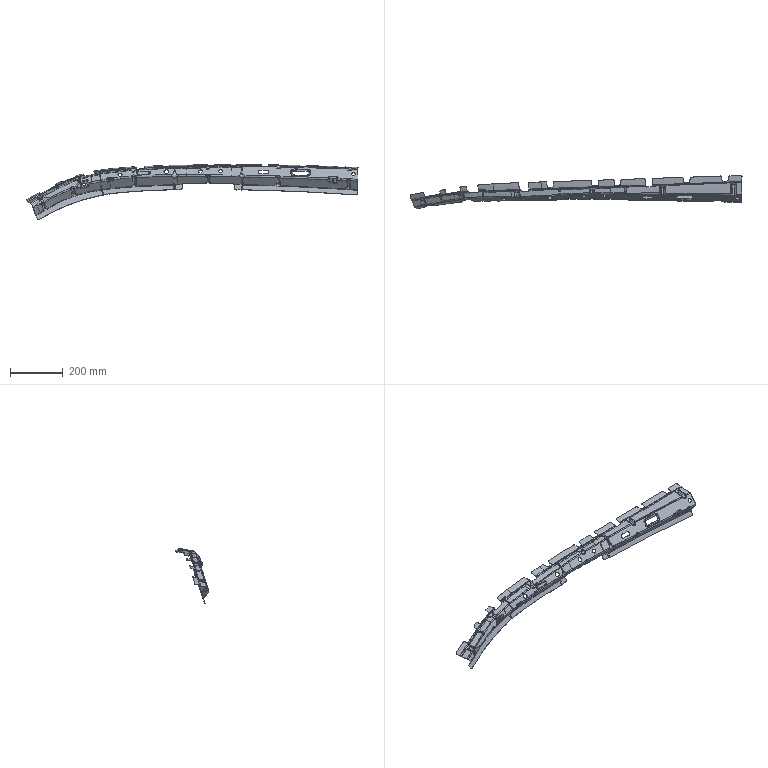Part | STEP file | FNA5401171 | 1 solid | 1265 faces | box 1257 x 126.52 x 207.673 mm | volume 214669 mm3 | spline 1123 | plane 60 | cylinder 34 | sphere 32 | other 16 | commonest cylinder face diameters 10 x8 8 x7 5.6 x3 7.6 x3 12.4 x3 12 x2